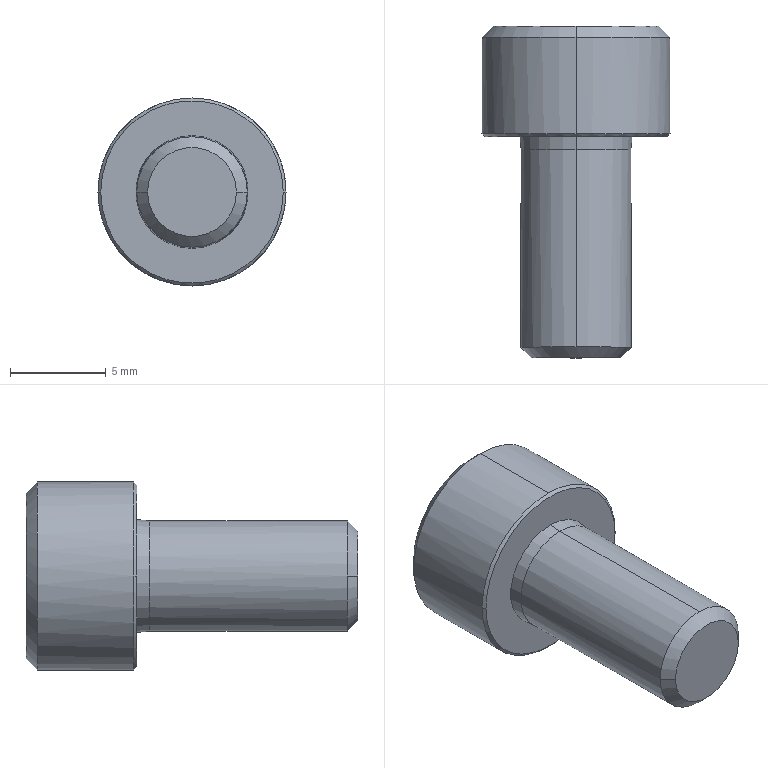Part | SolidWorks | features BaseBody 1 | 1 solid | 36 faces | box 9.808 x 17.308 x 9.808 mm | volume 668.703 mm3 | cone 17 | plane 15 | cylinder 4 | commonest cylinder face diameters 5.769 x2 9.808 x2
STEP:
#1=CARTESIAN_POINT('',(187.694,195.028,223.717));
#2=VERTEX_POINT('',#1);
#3=CARTESIAN_POINT('',(184.809,195.028,220.832));
#4=VERTEX_POINT('',#3);
#5=CARTESIAN_POINT('',(184.809,195.028,223.717));
#6=DIRECTION('',(0.,1.,0.));
#7=DIRECTION('',(0.,0.,1.));
#8=AXIS2_PLACEMENT_3D('',#5,#6,#7);
#9=CIRCLE('',#8,2.885);
#10=EDGE_CURVE('',#2,#4,#9,.T.);
#11=ORIENTED_EDGE('',*,*,#10,.T.);
#12=CARTESIAN_POINT('',(184.809,205.308,220.832));
#13=VERTEX_POINT('',#12);
#14=CARTESIAN_POINT('',(184.809,194.462,220.832));
#15=DIRECTION('',(0.,1.,0.));
#16=VECTOR('',#15,1000.);
#17=LINE('',#14,#16);
#18=EDGE_CURVE('',#4,#13,#17,.T.);
#19=ORIENTED_EDGE('',*,*,#18,.T.);
#20=CARTESIAN_POINT('',(184.809,205.308,226.601));
#21=VERTEX_POINT('',#20);
#22=CARTESIAN_POINT('',(184.809,205.308,223.717));
#23=DIRECTION('',(0.,-1.,0.));
#24=DIRECTION('',(0.,0.,1.));
#25=AXIS2_PLACEMENT_3D('',#22,#23,#24);
#26=CIRCLE('',#25,2.885);
#27=EDGE_CURVE('',#13,#21,#26,.T.);
#28=ORIENTED_EDGE('',*,*,#27,.T.);
#29=CARTESIAN_POINT('',(184.809,195.028,226.601));
#30=VERTEX_POINT('',#29);
#31=CARTESIAN_POINT('',(184.809,194.462,226.601));
#32=DIRECTION('',(0.,1.,0.));
#33=VECTOR('',#32,1000.);
#34=LINE('',#31,#33);
#35=EDGE_CURVE('',#30,#21,#34,.T.);
#36=ORIENTED_EDGE('',*,*,#35,.F.);
#37=CARTESIAN_POINT('',(184.809,195.028,223.717));
#38=DIRECTION('',(0.,1.,0.));
#39=DIRECTION('',(0.,0.,1.));
#40=AXIS2_PLACEMENT_3D('',#37,#38,#39);
#41=CIRCLE('',#40,2.885);
#42=EDGE_CURVE('',#30,#2,#41,.T.);
#43=ORIENTED_EDGE('',*,*,#42,.T.);
#44=EDGE_LOOP('',(#11,#19,#28,#36,#43));
#45=FACE_OUTER_BOUND('',#44,.T.);
#46=CARTESIAN_POINT('',(184.809,194.462,223.717));
#47=DIRECTION('',(0.,1.,0.));
#48=DIRECTION('',(0.,0.,1.));
#49=AXIS2_PLACEMENT_3D('',#46,#47,#48);
#50=CYLINDRICAL_SURFACE('',#49,2.885);
#51=ADVANCED_FACE('',(#45),#50,.T.);
#52=CARTESIAN_POINT('',(182.491,194.462,223.717));
#53=VERTEX_POINT('',#52);
#54=CARTESIAN_POINT('',(187.128,194.462,223.717));
#55=VERTEX_POINT('',#54);
#56=CARTESIAN_POINT('',(184.809,194.462,223.717));
#57=DIRECTION('',(0.,1.,0.));
#58=DIRECTION('',(-1.,0.,0.));
#59=AXIS2_PLACEMENT_3D('',#56,#57,#58);
#60=CIRCLE('',#59,2.319);
#61=EDGE_CURVE('',#53,#55,#60,.T.);
#62=ORIENTED_EDGE('',*,*,#61,.T.);
#63=CARTESIAN_POINT('',(187.694,195.028,223.717));
#64=DIRECTION('',(0.7071,0.7071,0.));
#65=VECTOR('',#64,1000.);
#66=LINE('',#63,#65);
#67=EDGE_CURVE('',#55,#2,#66,.T.);
#68=ORIENTED_EDGE('',*,*,#67,.T.);
#69=ORIENTED_EDGE('',*,*,#42,.F.);
#70=CARTESIAN_POINT('',(181.925,195.028,223.717));
#71=VERTEX_POINT('',#70);
#72=CARTESIAN_POINT('',(184.809,195.028,223.717));
#73=DIRECTION('',(0.,1.,0.));
#74=DIRECTION('',(0.,0.,1.));
#75=AXIS2_PLACEMENT_3D('',#72,#73,#74);
#76=CIRCLE('',#75,2.885);
#77=EDGE_CURVE('',#71,#30,#76,.T.);
#78=ORIENTED_EDGE('',*,*,#77,.F.);
#79=CARTESIAN_POINT('',(181.925,195.028,223.717));
#80=DIRECTION('',(-0.7071,0.7071,0.));
#81=VECTOR('',#80,1000.);
#82=LINE('',#79,#81);
#83=EDGE_CURVE('',#53,#71,#82,.T.);
#84=ORIENTED_EDGE('',*,*,#83,.F.);
#85=EDGE_LOOP('',(#62,#68,#69,#78,#84));
#86=FACE_OUTER_BOUND('',#85,.T.);
#87=CARTESIAN_POINT('',(184.809,195.028,223.717));
#88=DIRECTION('',(0.,1.,0.));
#89=DIRECTION('',(-1.,0.,0.));
#90=AXIS2_PLACEMENT_3D('',#87,#88,#89);
#91=CONICAL_SURFACE('',#90,2.885,0.7854);
#92=ADVANCED_FACE('',(#86),#91,.T.);
#93=ORIENTED_EDGE('',*,*,#27,.F.);
#94=CARTESIAN_POINT('',(184.809,206.,220.774));
#95=VERTEX_POINT('',#94);
#96=CARTESIAN_POINT('',(184.809,206.,220.774));
#97=DIRECTION('',(0.,0.9965,-0.08305));
#98=VECTOR('',#97,1000.);
#99=LINE('',#96,#98);
#100=EDGE_CURVE('',#13,#95,#99,.T.);
#101=ORIENTED_EDGE('',*,*,#100,.T.);
#102=CARTESIAN_POINT('',(184.809,206.,226.659));
#103=VERTEX_POINT('',#102);
#104=CARTESIAN_POINT('',(184.809,206.,223.717));
#105=DIRECTION('',(0.,-1.,0.));
#106=DIRECTION('',(0.,0.,1.));
#107=AXIS2_PLACEMENT_3D('',#104,#105,#106);
#108=CIRCLE('',#107,2.942);
#109=EDGE_CURVE('',#95,#103,#108,.T.);
#110=ORIENTED_EDGE('',*,*,#109,.T.);
#111=CARTESIAN_POINT('',(184.809,206.,226.659));
#112=DIRECTION('',(0.,0.9965,0.08305));
#113=VECTOR('',#112,1000.);
#114=LINE('',#111,#113);
#115=EDGE_CURVE('',#21,#103,#114,.T.);
#116=ORIENTED_EDGE('',*,*,#115,.F.);
#117=EDGE_LOOP('',(#93,#101,#110,#116));
#118=FACE_OUTER_BOUND('',#117,.T.);
#119=CARTESIAN_POINT('',(184.809,206.,223.717));
#120=DIRECTION('',(0.,1.,0.));
#121=DIRECTION('',(0.,0.,1.));
#122=AXIS2_PLACEMENT_3D('',#119,#120,#121);
#123=CONICAL_SURFACE('',#122,2.942,0.08314);
#124=ADVANCED_FACE('',(#118),#123,.T.);
#125=CARTESIAN_POINT('',(180.05,206.,223.717));
#126=VERTEX_POINT('',#125);
#127=CARTESIAN_POINT('',(189.569,206.,223.717));
#128=VERTEX_POINT('',#127);
#129=CARTESIAN_POINT('',(184.809,206.,223.717));
#130=DIRECTION('',(0.,1.,0.));
#131=DIRECTION('',(-1.,0.,0.));
#132=AXIS2_PLACEMENT_3D('',#129,#130,#131);
#133=CIRCLE('',#132,4.76);
#134=EDGE_CURVE('',#126,#128,#133,.T.);
#135=ORIENTED_EDGE('',*,*,#134,.T.);
#136=CARTESIAN_POINT('',(189.713,206.144,223.717));
#137=VERTEX_POINT('',#136);
#138=CARTESIAN_POINT('',(189.713,206.144,223.717));
#139=DIRECTION('',(0.7071,0.7071,0.));
#140=VECTOR('',#139,1000.);
#141=LINE('',#138,#140);
#142=EDGE_CURVE('',#128,#137,#141,.T.);
#143=ORIENTED_EDGE('',*,*,#142,.T.);
#144=CARTESIAN_POINT('',(184.809,206.144,228.621));
#145=VERTEX_POINT('',#144);
#146=CARTESIAN_POINT('',(184.809,206.144,223.717));
#147=DIRECTION('',(0.,-1.,0.));
#148=DIRECTION('',(0.,0.,-1.));
#149=AXIS2_PLACEMENT_3D('',#146,#147,#148);
#150=CIRCLE('',#149,4.904);
#151=EDGE_CURVE('',#137,#145,#150,.T.);
#152=ORIENTED_EDGE('',*,*,#151,.T.);
#153=CARTESIAN_POINT('',(179.906,206.144,223.717));
#154=VERTEX_POINT('',#153);
#155=CARTESIAN_POINT('',(184.809,206.144,223.717));
#156=DIRECTION('',(0.,-1.,0.));
#157=DIRECTION('',(0.,0.,-1.));
#158=AXIS2_PLACEMENT_3D('',#155,#156,#157);
#159=CIRCLE('',#158,4.904);
#160=EDGE_CURVE('',#145,#154,#159,.T.);
#161=ORIENTED_EDGE('',*,*,#160,.T.);
#162=CARTESIAN_POINT('',(179.906,206.144,223.717));
#163=DIRECTION('',(-0.7071,0.7071,0.));
#164=VECTOR('',#163,1000.);
#165=LINE('',#162,#164);
#166=EDGE_CURVE('',#126,#154,#165,.T.);
#167=ORIENTED_EDGE('',*,*,#166,.F.);
#168=EDGE_LOOP('',(#135,#143,#152,#161,#167));
#169=FACE_OUTER_BOUND('',#168,.T.);
#170=CARTESIAN_POINT('',(184.809,206.144,223.717));
#171=DIRECTION('',(0.,1.,0.));
#172=DIRECTION('',(-1.,0.,0.));
#173=AXIS2_PLACEMENT_3D('',#170,#171,#172);
#174=CONICAL_SURFACE('',#173,4.904,0.7854);
#175=ADVANCED_FACE('',(#169),#174,.T.);
#176=CARTESIAN_POINT('',(184.809,206.144,218.813));
#177=VERTEX_POINT('',#176);
#178=CARTESIAN_POINT('',(184.809,206.144,223.717));
#179=DIRECTION('',(0.,-1.,0.));
#180=DIRECTION('',(0.,0.,-1.));
#181=AXIS2_PLACEMENT_3D('',#178,#179,#180);
#182=CIRCLE('',#181,4.904);
#183=EDGE_CURVE('',#177,#137,#182,.T.);
#184=ORIENTED_EDGE('',*,*,#183,.F.);
#185=CARTESIAN_POINT('',(184.809,211.192,218.813));
#186=VERTEX_POINT('',#185);
#187=CARTESIAN_POINT('',(184.809,194.462,218.813));
#188=DIRECTION('',(0.,1.,0.));
#189=VECTOR('',#188,1000.);
#190=LINE('',#187,#189);
#191=EDGE_CURVE('',#177,#186,#190,.T.);
#192=ORIENTED_EDGE('',*,*,#191,.T.);
#193=CARTESIAN_POINT('',(184.809,211.192,228.621));
#194=VERTEX_POINT('',#193);
#195=CARTESIAN_POINT('',(184.809,211.192,223.717));
#196=DIRECTION('',(0.,-1.,0.));
#197=DIRECTION('',(0.,0.,1.));
#198=AXIS2_PLACEMENT_3D('',#195,#196,#197);
#199=CIRCLE('',#198,4.904);
#200=EDGE_CURVE('',#186,#194,#199,.T.);
#201=ORIENTED_EDGE('',*,*,#200,.T.);
#202=CARTESIAN_POINT('',(184.809,194.462,228.621));
#203=DIRECTION('',(0.,1.,0.));
#204=VECTOR('',#203,1000.);
#205=LINE('',#202,#204);
#206=EDGE_CURVE('',#145,#194,#205,.T.);
#207=ORIENTED_EDGE('',*,*,#206,.F.);
#208=ORIENTED_EDGE('',*,*,#151,.F.);
#209=EDGE_LOOP('',(#184,#192,#201,#207,#208));
#210=FACE_OUTER_BOUND('',#209,.T.);
#211=CARTESIAN_POINT('',(184.809,194.462,223.717));
#212=DIRECTION('',(0.,1.,0.));
#213=DIRECTION('',(0.,0.,1.));
#214=AXIS2_PLACEMENT_3D('',#211,#212,#213);
#215=CYLINDRICAL_SURFACE('',#214,4.904);
#216=ADVANCED_FACE('',(#210),#215,.T.);
#217=CARTESIAN_POINT('',(184.809,211.769,219.39));
#218=VERTEX_POINT('',#217);
#219=CARTESIAN_POINT('',(184.809,211.769,228.044));
#220=VERTEX_POINT('',#219);
#221=CARTESIAN_POINT('',(184.809,211.769,223.717));
#222=DIRECTION('',(0.,-1.,0.));
#223=DIRECTION('',(0.,0.,-1.));
#224=AXIS2_PLACEMENT_3D('',#221,#222,#223);
#225=CIRCLE('',#224,4.327);
#226=EDGE_CURVE('',#218,#220,#225,.T.);
#227=ORIENTED_EDGE('',*,*,#226,.T.);
#228=CARTESIAN_POINT('',(184.809,211.192,228.621));
#229=DIRECTION('',(0.,-0.7071,0.7071));
#230=VECTOR('',#229,1000.);
#231=LINE('',#228,#230);
#232=EDGE_CURVE('',#220,#194,#231,.T.);
#233=ORIENTED_EDGE('',*,*,#232,.T.);
#234=ORIENTED_EDGE('',*,*,#200,.F.);
#235=CARTESIAN_POINT('',(184.809,211.192,218.813));
#236=DIRECTION('',(0.,-0.7071,-0.7071));
#237=VECTOR('',#236,1000.);
#238=LINE('',#235,#237);
#239=EDGE_CURVE('',#218,#186,#238,.T.);
#240=ORIENTED_EDGE('',*,*,#239,.F.);
#241=EDGE_LOOP('',(#227,#233,#234,#240));
#242=FACE_OUTER_BOUND('',#241,.T.);
#243=CARTESIAN_POINT('',(184.809,211.192,223.717));
#244=DIRECTION('',(0.,-1.,0.));
#245=DIRECTION('',(0.,0.,-1.));
#246=AXIS2_PLACEMENT_3D('',#243,#244,#245);
#247=CONICAL_SURFACE('',#246,4.904,0.7854);
#248=ADVANCED_FACE('',(#242),#247,.T.);
#249=CARTESIAN_POINT('',(182.502,211.412,223.717));
#250=VERTEX_POINT('',#249);
#251=CARTESIAN_POINT('',(182.502,211.769,225.049));
#252=VERTEX_POINT('',#251);
#253=CARTESIAN_POINT('',(182.502,211.412,223.717));
#254=CARTESIAN_POINT('',(182.502,211.412,223.949));
#255=CARTESIAN_POINT('',(182.502,211.448,224.176));
#256=CARTESIAN_POINT('',(182.502,211.575,224.626));
#257=CARTESIAN_POINT('',(182.502,211.665,224.84));
#258=CARTESIAN_POINT('',(182.502,211.769,225.049));
#259=B_SPLINE_CURVE_WITH_KNOTS('',3,(#253,#254,#255,#256,#257,#258),.UNSPECIFIED.,.F.,.F.,(4,2,4),(0.001381,0.002067,0.002753),.UNSPECIFIED.);
#260=EDGE_CURVE('',#250,#252,#259,.T.);
#261=ORIENTED_EDGE('',*,*,#260,.F.);
#262=CARTESIAN_POINT('',(182.145,211.769,223.717));
#263=VERTEX_POINT('',#262);
#264=CARTESIAN_POINT('',(182.145,211.769,223.717));
#265=DIRECTION('',(-0.7071,0.7071,0.));
#266=VECTOR('',#265,1000.);
#267=LINE('',#264,#266);
#268=EDGE_CURVE('',#250,#263,#267,.T.);
#269=ORIENTED_EDGE('',*,*,#268,.T.);
#270=CARTESIAN_POINT('',(184.809,211.769,223.717));
#271=DIRECTION('',(0.,1.,0.));
#272=DIRECTION('',(-1.,0.,0.));
#273=AXIS2_PLACEMENT_3D('',#270,#271,#272);
#274=CIRCLE('',#273,2.665);
#275=EDGE_CURVE('',#263,#252,#274,.T.);
#276=ORIENTED_EDGE('',*,*,#275,.T.);
#277=EDGE_LOOP('',(#261,#269,#276));
#278=FACE_OUTER_BOUND('',#277,.T.);
#279=CARTESIAN_POINT('',(184.809,211.769,223.717));
#280=DIRECTION('',(0.,1.,0.));
#281=DIRECTION('',(-1.,0.,0.));
#282=AXIS2_PLACEMENT_3D('',#279,#280,#281);
#283=CONICAL_SURFACE('',#282,2.665,0.7854);
#284=ADVANCED_FACE('',(#278),#283,.F.);
#285=CARTESIAN_POINT('',(184.809,207.552,223.717));
#286=VERTEX_POINT('',#285);
#287=CARTESIAN_POINT('',(182.502,208.885,223.717));
#288=VERTEX_POINT('',#287);
#289=CARTESIAN_POINT('',(182.502,208.885,223.717));
#290=DIRECTION('',(-0.866,0.5,0.));
#291=VECTOR('',#290,1000.);
#292=LINE('',#289,#291);
#293=EDGE_CURVE('',#286,#288,#292,.T.);
#294=ORIENTED_EDGE('',*,*,#293,.F.);
#295=CARTESIAN_POINT('',(187.117,208.885,223.717));
#296=VERTEX_POINT('',#295);
#297=CARTESIAN_POINT('',(187.117,208.885,223.717));
#298=DIRECTION('',(0.866,0.5,0.));
#299=VECTOR('',#298,1000.);
#300=LINE('',#297,#299);
#301=EDGE_CURVE('',#286,#296,#300,.T.);
#302=ORIENTED_EDGE('',*,*,#301,.T.);
#303=CARTESIAN_POINT('',(185.963,208.885,221.718));
#304=VERTEX_POINT('',#303);
#305=CARTESIAN_POINT('',(184.809,208.885,223.717));
#306=DIRECTION('',(0.,-1.,0.));
#307=DIRECTION('',(-1.,0.,0.));
#308=AXIS2_PLACEMENT_3D('',#305,#306,#307);
#309=CIRCLE('',#308,2.308);
#310=EDGE_CURVE('',#304,#296,#309,.T.);
#311=ORIENTED_EDGE('',*,*,#310,.F.);
#312=CARTESIAN_POINT('',(183.656,208.885,221.718));
#313=VERTEX_POINT('',#312);
#314=CARTESIAN_POINT('',(184.809,208.885,223.717));
#315=DIRECTION('',(0.,-1.,0.));
#316=DIRECTION('',(-1.,0.,0.));
#317=AXIS2_PLACEMENT_3D('',#314,#315,#316);
#318=CIRCLE('',#317,2.308);
#319=EDGE_CURVE('',#313,#304,#318,.T.);
#320=ORIENTED_EDGE('',*,*,#319,.F.);
#321=CARTESIAN_POINT('',(184.809,208.885,223.717));
#322=DIRECTION('',(0.,-1.,0.));
#323=DIRECTION('',(0.,0.,1.));
#324=AXIS2_PLACEMENT_3D('',#321,#322,#323);
#325=CIRCLE('',#324,2.308);
#326=EDGE_CURVE('',#288,#313,#325,.T.);
#327=ORIENTED_EDGE('',*,*,#326,.F.);
#328=EDGE_LOOP('',(#294,#302,#311,#320,#327));
#329=FACE_OUTER_BOUND('',#328,.T.);
#330=CARTESIAN_POINT('',(184.809,208.885,223.717));
#331=DIRECTION('',(0.,1.,0.));
#332=DIRECTION('',(-1.,0.,0.));
#333=AXIS2_PLACEMENT_3D('',#330,#331,#332);
#334=CONICAL_SURFACE('',#333,2.308,1.047);
#335=ADVANCED_FACE('',(#329),#334,.F.);
#336=ORIENTED_EDGE('',*,*,#18,.F.);
#337=CARTESIAN_POINT('',(184.809,195.028,223.717));
#338=DIRECTION('',(0.,1.,0.));
#339=DIRECTION('',(0.,0.,1.));
#340=AXIS2_PLACEMENT_3D('',#337,#338,#339);
#341=CIRCLE('',#340,2.885);
#342=EDGE_CURVE('',#4,#71,#341,.T.);
#343=ORIENTED_EDGE('',*,*,#342,.T.);
#344=ORIENTED_EDGE('',*,*,#77,.T.);
#345=ORIENTED_EDGE('',*,*,#35,.T.);
#346=CARTESIAN_POINT('',(184.809,205.308,223.717));
#347=DIRECTION('',(0.,-1.,0.));
#348=DIRECTION('',(0.,0.,1.));
#349=AXIS2_PLACEMENT_3D('',#346,#347,#348);
#350=CIRCLE('',#349,2.885);
#351=EDGE_CURVE('',#21,#13,#350,.T.);
#352=ORIENTED_EDGE('',*,*,#351,.T.);
#353=EDGE_LOOP('',(#336,#343,#344,#345,#352));
#354=FACE_OUTER_BOUND('',#353,.T.);
#355=CARTESIAN_POINT('',(184.809,194.462,223.717));
#356=DIRECTION('',(0.,1.,0.));
#357=DIRECTION('',(0.,0.,1.));
#358=AXIS2_PLACEMENT_3D('',#355,#356,#357);
#359=CYLINDRICAL_SURFACE('',#358,2.885);
#360=ADVANCED_FACE('',(#354),#359,.T.);
#361=ORIENTED_EDGE('',*,*,#67,.F.);
#362=CARTESIAN_POINT('',(184.809,194.462,223.717));
#363=DIRECTION('',(0.,1.,0.));
#364=DIRECTION('',(-1.,0.,0.));
#365=AXIS2_PLACEMENT_3D('',#362,#363,#364);
#366=CIRCLE('',#365,2.319);
#367=EDGE_CURVE('',#55,#53,#366,.T.);
#368=ORIENTED_EDGE('',*,*,#367,.T.);
#369=ORIENTED_EDGE('',*,*,#83,.T.);
#370=ORIENTED_EDGE('',*,*,#342,.F.);
#371=ORIENTED_EDGE('',*,*,#10,.F.);
#372=EDGE_LOOP('',(#361,#368,#369,#370,#371));
#373=FACE_OUTER_BOUND('',#372,.T.);
#374=CARTESIAN_POINT('',(184.809,195.028,223.717));
#375=DIRECTION('',(0.,1.,0.));
#376=DIRECTION('',(-1.,0.,0.));
#377=AXIS2_PLACEMENT_3D('',#374,#375,#376);
#378=CONICAL_SURFACE('',#377,2.885,0.7854);
#379=ADVANCED_FACE('',(#373),#378,.T.);
#380=ORIENTED_EDGE('',*,*,#100,.F.);
#381=ORIENTED_EDGE('',*,*,#351,.F.);
#382=ORIENTED_EDGE('',*,*,#115,.T.);
#383=CARTESIAN_POINT('',(184.809,206.,223.717));
#384=DIRECTION('',(0.,-1.,0.));
#385=DIRECTION('',(0.,0.,1.));
#386=AXIS2_PLACEMENT_3D('',#383,#384,#385);
#387=CIRCLE('',#386,2.942);
#388=EDGE_CURVE('',#103,#95,#387,.T.);
#389=ORIENTED_EDGE('',*,*,#388,.T.);
#390=EDGE_LOOP('',(#380,#381,#382,#389));
#391=FACE_OUTER_BOUND('',#390,.T.);
#392=CARTESIAN_POINT('',(184.809,206.,223.717));
#393=DIRECTION('',(0.,1.,0.));
#394=DIRECTION('',(0.,0.,1.));
#395=AXIS2_PLACEMENT_3D('',#392,#393,#394);
#396=CONICAL_SURFACE('',#395,2.942,0.08314);
#397=ADVANCED_FACE('',(#391),#396,.T.);
#398=ORIENTED_EDGE('',*,*,#61,.F.);
#399=ORIENTED_EDGE('',*,*,#367,.F.);
#400=EDGE_LOOP('',(#398,#399));
#401=FACE_OUTER_BOUND('',#400,.T.);
#402=CARTESIAN_POINT('',(187.128,194.462,223.717));
#403=DIRECTION('',(0.,1.,0.));
#404=DIRECTION('',(0.,0.,1.));
#405=AXIS2_PLACEMENT_3D('',#402,#403,#404);
#406=PLANE('',#405);
#407=ADVANCED_FACE('',(#401),#406,.F.);
#408=ORIENTED_EDGE('',*,*,#388,.F.);
#409=ORIENTED_EDGE('',*,*,#109,.F.);
#410=EDGE_LOOP('',(#408,#409));
#411=FACE_BOUND('',#410,.T.);
#412=ORIENTED_EDGE('',*,*,#134,.F.);
#413=CARTESIAN_POINT('',(184.809,206.,223.717));
#414=DIRECTION('',(0.,1.,0.));
#415=DIRECTION('',(-1.,0.,0.));
#416=AXIS2_PLACEMENT_3D('',#413,#414,#415);
#417=CIRCLE('',#416,4.76);
#418=EDGE_CURVE('',#128,#126,#417,.T.);
#419=ORIENTED_EDGE('',*,*,#418,.F.);
#420=EDGE_LOOP('',(#412,#419));
#421=FACE_OUTER_BOUND('',#420,.T.);
#422=CARTESIAN_POINT('',(189.569,206.,223.717));
#423=DIRECTION('',(0.,1.,0.));
#424=DIRECTION('',(0.,0.,1.));
#425=AXIS2_PLACEMENT_3D('',#422,#423,#424);
#426=PLANE('',#425);
#427=ADVANCED_FACE('',(#411,#421),#426,.F.);
#428=ORIENTED_EDGE('',*,*,#142,.F.);
#429=ORIENTED_EDGE('',*,*,#418,.T.);
#430=ORIENTED_EDGE('',*,*,#166,.T.);
#431=CARTESIAN_POINT('',(184.809,206.144,223.717));
#432=DIRECTION('',(0.,-1.,0.));
#433=DIRECTION('',(0.,0.,-1.));
#434=AXIS2_PLACEMENT_3D('',#431,#432,#433);
#435=CIRCLE('',#434,4.904);
#436=EDGE_CURVE('',#154,#177,#435,.T.);
#437=ORIENTED_EDGE('',*,*,#436,.T.);
#438=ORIENTED_EDGE('',*,*,#183,.T.);
#439=EDGE_LOOP('',(#428,#429,#430,#437,#438));
#440=FACE_OUTER_BOUND('',#439,.T.);
#441=CARTESIAN_POINT('',(184.809,206.144,223.717));
#442=DIRECTION('',(0.,1.,0.));
#443=DIRECTION('',(-1.,0.,0.));
#444=AXIS2_PLACEMENT_3D('',#441,#442,#443);
#445=CONICAL_SURFACE('',#444,4.904,0.7854);
#446=ADVANCED_FACE('',(#440),#445,.T.);
#447=ORIENTED_EDGE('',*,*,#191,.F.);
#448=ORIENTED_EDGE('',*,*,#436,.F.);
#449=ORIENTED_EDGE('',*,*,#160,.F.);
#450=ORIENTED_EDGE('',*,*,#206,.T.);
#451=CARTESIAN_POINT('',(184.809,211.192,223.717));
#452=DIRECTION('',(0.,-1.,0.));
#453=DIRECTION('',(0.,0.,1.));
#454=AXIS2_PLACEMENT_3D('',#451,#452,#453);
#455=CIRCLE('',#454,4.904);
#456=EDGE_CURVE('',#194,#186,#455,.T.);
#457=ORIENTED_EDGE('',*,*,#456,.T.);
#458=EDGE_LOOP('',(#447,#448,#449,#450,#457));
#459=FACE_OUTER_BOUND('',#458,.T.);
#460=CARTESIAN_POINT('',(184.809,194.462,223.717));
#461=DIRECTION('',(0.,1.,0.));
#462=DIRECTION('',(0.,0.,1.));
#463=AXIS2_PLACEMENT_3D('',#460,#461,#462);
#464=CYLINDRICAL_SURFACE('',#463,4.904);
#465=ADVANCED_FACE('',(#459),#464,.T.);
#466=ORIENTED_EDGE('',*,*,#232,.F.);
#467=CARTESIAN_POINT('',(184.809,211.769,223.717));
#468=DIRECTION('',(0.,-1.,0.));
#469=DIRECTION('',(0.,0.,-1.));
#470=AXIS2_PLACEMENT_3D('',#467,#468,#469);
#471=CIRCLE('',#470,4.327);
#472=EDGE_CURVE('',#220,#218,#471,.T.);
#473=ORIENTED_EDGE('',*,*,#472,.T.);
#474=ORIENTED_EDGE('',*,*,#239,.T.);
#475=ORIENTED_EDGE('',*,*,#456,.F.);
#476=EDGE_LOOP('',(#466,#473,#474,#475));
#477=FACE_OUTER_BOUND('',#476,.T.);
#478=CARTESIAN_POINT('',(184.809,211.192,223.717));
#479=DIRECTION('',(0.,-1.,0.));
#480=DIRECTION('',(0.,0.,-1.));
#481=AXIS2_PLACEMENT_3D('',#478,#479,#480);
#482=CONICAL_SURFACE('',#481,4.904,0.7854);
#483=ADVANCED_FACE('',(#477),#482,.T.);
#484=CARTESIAN_POINT('',(184.809,211.769,226.381));
#485=VERTEX_POINT('',#484);
#486=CARTESIAN_POINT('',(184.809,211.769,223.717));
#487=DIRECTION('',(0.,1.,0.));
#488=DIRECTION('',(-1.,0.,0.));
#489=AXIS2_PLACEMENT_3D('',#486,#487,#488);
#490=CIRCLE('',#489,2.665);
#491=EDGE_CURVE('',#252,#485,#490,.T.);
#492=ORIENTED_EDGE('',*,*,#491,.F.);
#493=ORIENTED_EDGE('',*,*,#275,.F.);
#494=CARTESIAN_POINT('',(182.502,211.769,222.384));
#495=VERTEX_POINT('',#494);
#496=CARTESIAN_POINT('',(184.809,211.769,223.717));
#497=DIRECTION('',(0.,1.,0.));
#498=DIRECTION('',(-1.,0.,0.));
#499=AXIS2_PLACEMENT_3D('',#496,#497,#498);
#500=CIRCLE('',#499,2.665);
#501=EDGE_CURVE('',#495,#263,#500,.T.);
#502=ORIENTED_EDGE('',*,*,#501,.F.);
#503=CARTESIAN_POINT('',(184.809,211.769,221.052));
#504=VERTEX_POINT('',#503);
#505=CARTESIAN_POINT('',(184.809,211.769,223.717));
#506=DIRECTION('',(0.,1.,0.));
#507=DIRECTION('',(0.,0.,1.));
#508=AXIS2_PLACEMENT_3D('',#505,#506,#507);
#509=CIRCLE('',#508,2.665);
#510=EDGE_CURVE('',#504,#495,#509,.T.);
#511=ORIENTED_EDGE('',*,*,#510,.F.);
#512=CARTESIAN_POINT('',(187.117,211.769,222.384));
#513=VERTEX_POINT('',#512);
#514=CARTESIAN_POINT('',(184.809,211.769,223.717));
#515=DIRECTION('',(0.,1.,0.));
#516=DIRECTION('',(0.,0.,1.));
#517=AXIS2_PLACEMENT_3D('',#514,#515,#516);
#518=CIRCLE('',#517,2.665);
#519=EDGE_CURVE('',#513,#504,#518,.T.);
#520=ORIENTED_EDGE('',*,*,#519,.F.);
#521=CARTESIAN_POINT('',(187.117,211.769,225.049));
#522=VERTEX_POINT('',#521);
#523=CARTESIAN_POINT('',(184.809,211.769,223.717));
#524=DIRECTION('',(0.,1.,0.));
#525=DIRECTION('',(0.,0.,1.));
#526=AXIS2_PLACEMENT_3D('',#523,#524,#525);
#527=CIRCLE('',#526,2.665);
#528=EDGE_CURVE('',#522,#513,#527,.T.);
#529=ORIENTED_EDGE('',*,*,#528,.F.);
#530=CARTESIAN_POINT('',(184.809,211.769,223.717));
#531=DIRECTION('',(0.,1.,0.));
#532=DIRECTION('',(0.,0.,1.));
#533=AXIS2_PLACEMENT_3D('',#530,#531,#532);
#534=CIRCLE('',#533,2.665);
#535=EDGE_CURVE('',#485,#522,#534,.T.);
#536=ORIENTED_EDGE('',*,*,#535,.F.);
#537=EDGE_LOOP('',(#492,#493,#502,#511,#520,#529,#536));
#538=FACE_BOUND('',#537,.T.);
#539=ORIENTED_EDGE('',*,*,#226,.F.);
#540=ORIENTED_EDGE('',*,*,#472,.F.);
#541=EDGE_LOOP('',(#539,#540));
#542=FACE_OUTER_BOUND('',#541,.T.);
#543=CARTESIAN_POINT('',(187.474,211.769,223.717));
#544=DIRECTION('',(0.,-1.,0.));
#545=DIRECTION('',(0.,0.,-1.));
#546=AXIS2_PLACEMENT_3D('',#543,#544,#545);
#547=PLANE('',#546);
#548=ADVANCED_FACE('',(#538,#542),#547,.F.);
#549=CARTESIAN_POINT('',(184.809,211.769,226.381));
#550=CARTESIAN_POINT('',(184.99,211.665,226.277));
#551=CARTESIAN_POINT('',(185.174,211.577,226.171));
#552=CARTESIAN_POINT('',(185.461,211.482,226.006));
#553=CARTESIAN_POINT('',(185.558,211.457,225.949));
#554=CARTESIAN_POINT('',(185.756,211.422,225.835));
#555=CARTESIAN_POINT('',(185.858,211.413,225.776));
#556=CARTESIAN_POINT('',(186.161,211.412,225.601));
#557=CARTESIAN_POINT('',(186.359,211.447,225.487));
#558=CARTESIAN_POINT('',(186.749,211.575,225.262));
#559=CARTESIAN_POINT('',(186.936,211.665,225.154));
#560=CARTESIAN_POINT('',(187.117,211.769,225.049));
#561=B_SPLINE_CURVE_WITH_KNOTS('',3,(#549,#550,#551,#552,#553,#554,#555,#556,#557,#558,#559,#560),.UNSPECIFIED.,.F.,.F.,(4,2,2,2,2,4),(0.,0.0006881,0.001032,0.001376,0.002064,0.002753),.UNSPECIFIED.);
#562=EDGE_CURVE('',#485,#522,#561,.T.);
#563=ORIENTED_EDGE('',*,*,#562,.F.);
#564=ORIENTED_EDGE('',*,*,#535,.T.);
#565=EDGE_LOOP('',(#563,#564));
#566=FACE_OUTER_BOUND('',#565,.T.);
#567=CARTESIAN_POINT('',(184.809,211.769,223.717));
#568=DIRECTION('',(0.,1.,0.));
#569=DIRECTION('',(0.,0.,1.));
#570=AXIS2_PLACEMENT_3D('',#567,#568,#569);
#571=CONICAL_SURFACE('',#570,2.665,0.7854);
#572=ADVANCED_FACE('',(#566),#571,.F.);
#573=CARTESIAN_POINT('',(182.502,211.769,225.049));
#574=CARTESIAN_POINT('',(182.682,211.665,225.153));
#575=CARTESIAN_POINT('',(182.866,211.577,225.26));
#576=CARTESIAN_POINT('',(183.153,211.482,225.425));
#577=CARTESIAN_POINT('',(183.25,211.457,225.481));
#578=CARTESIAN_POINT('',(183.448,211.422,225.596));
#579=CARTESIAN_POINT('',(183.551,211.413,225.655));
#580=CARTESIAN_POINT('',(183.853,211.412,225.829));
#581=CARTESIAN_POINT('',(184.051,211.447,225.944));
#582=CARTESIAN_POINT('',(184.441,211.575,226.169));
#583=CARTESIAN_POINT('',(184.628,211.665,226.277));
#584=CARTESIAN_POINT('',(184.809,211.769,226.381));
#585=B_SPLINE_CURVE_WITH_KNOTS('',3,(#573,#574,#575,#576,#577,#578,#579,#580,#581,#582,#583,#584),.UNSPECIFIED.,.F.,.F.,(4,2,2,2,2,4),(0.,0.0006881,0.001032,0.001376,0.002064,0.002753),.UNSPECIFIED.);
#586=EDGE_CURVE('',#252,#485,#585,.T.);
#587=ORIENTED_EDGE('',*,*,#586,.F.);
#588=ORIENTED_EDGE('',*,*,#491,.T.);
#589=EDGE_LOOP('',(#587,#588));
#590=FACE_OUTER_BOUND('',#589,.T.);
#591=CARTESIAN_POINT('',(184.809,211.769,223.717));
#592=DIRECTION('',(0.,1.,0.));
#593=DIRECTION('',(-1.,0.,0.));
#594=AXIS2_PLACEMENT_3D('',#591,#592,#593);
#595=CONICAL_SURFACE('',#594,2.665,0.7854);
#596=ADVANCED_FACE('',(#590),#595,.F.);
#597=ORIENTED_EDGE('',*,*,#268,.F.);
#598=CARTESIAN_POINT('',(182.502,211.769,222.384));
#599=CARTESIAN_POINT('',(182.502,211.665,222.593));
#600=CARTESIAN_POINT('',(182.502,211.576,222.807));
#601=CARTESIAN_POINT('',(182.502,211.481,223.139));
#602=CARTESIAN_POINT('',(182.502,211.456,223.252));
#603=CARTESIAN_POINT('',(182.502,211.421,223.482));
#604=CARTESIAN_POINT('',(182.502,211.412,223.6));
#605=CARTESIAN_POINT('',(182.502,211.412,223.717));
#606=B_SPLINE_CURVE_WITH_KNOTS('',3,(#598,#599,#600,#601,#602,#603,#604,#605),.UNSPECIFIED.,.F.,.F.,(4,2,2,4),(0.,0.0006905,0.001036,0.001381),.UNSPECIFIED.);
#607=EDGE_CURVE('',#495,#250,#606,.T.);
#608=ORIENTED_EDGE('',*,*,#607,.F.);
#609=ORIENTED_EDGE('',*,*,#501,.T.);
#610=EDGE_LOOP('',(#597,#608,#609));
#611=FACE_OUTER_BOUND('',#610,.T.);
#612=CARTESIAN_POINT('',(184.809,211.769,223.717));
#613=DIRECTION('',(0.,1.,0.));
#614=DIRECTION('',(-1.,0.,0.));
#615=AXIS2_PLACEMENT_3D('',#612,#613,#614);
#616=CONICAL_SURFACE('',#615,2.665,0.7854);
#617=ADVANCED_FACE('',(#611),#616,.F.);
#618=CARTESIAN_POINT('',(184.809,211.769,221.052));
#619=CARTESIAN_POINT('',(184.629,211.665,221.156));
#620=CARTESIAN_POINT('',(184.445,211.577,221.263));
#621=CARTESIAN_POINT('',(184.158,211.482,221.428));
#622=CARTESIAN_POINT('',(184.061,211.457,221.484));
#623=CARTESIAN_POINT('',(183.863,211.422,221.599));
#624=CARTESIAN_POINT('',(183.761,211.413,221.658));
#625=CARTESIAN_POINT('',(183.458,211.412,221.832));
#626=CARTESIAN_POINT('',(183.26,211.447,221.946));
#627=CARTESIAN_POINT('',(182.87,211.575,222.172));
#628=CARTESIAN_POINT('',(182.683,211.665,222.28));
#629=CARTESIAN_POINT('',(182.502,211.769,222.384));
#630=B_SPLINE_CURVE_WITH_KNOTS('',3,(#618,#619,#620,#621,#622,#623,#624,#625,#626,#627,#628,#629),.UNSPECIFIED.,.F.,.F.,(4,2,2,2,2,4),(0.,0.0006881,0.001032,0.001376,0.002064,0.002753),.UNSPECIFIED.);
#631=EDGE_CURVE('',#504,#495,#630,.T.);
#632=ORIENTED_EDGE('',*,*,#631,.F.);
#633=ORIENTED_EDGE('',*,*,#510,.T.);
#634=EDGE_LOOP('',(#632,#633));
#635=FACE_OUTER_BOUND('',#634,.T.);
#636=CARTESIAN_POINT('',(184.809,211.769,223.717));
#637=DIRECTION('',(0.,1.,0.));
#638=DIRECTION('',(0.,0.,1.));
#639=AXIS2_PLACEMENT_3D('',#636,#637,#638);
#640=CONICAL_SURFACE('',#639,2.665,0.7854);
#641=ADVANCED_FACE('',(#635),#640,.F.);
#642=CARTESIAN_POINT('',(187.117,211.769,222.384));
#643=CARTESIAN_POINT('',(186.937,211.665,222.28));
#644=CARTESIAN_POINT('',(186.752,211.577,222.174));
#645=CARTESIAN_POINT('',(186.466,211.482,222.009));
#646=CARTESIAN_POINT('',(186.369,211.457,221.952));
#647=CARTESIAN_POINT('',(186.17,211.422,221.838));
#648=CARTESIAN_POINT('',(186.068,211.413,221.779));
#649=CARTESIAN_POINT('',(185.766,211.412,221.604));
#650=CARTESIAN_POINT('',(185.568,211.447,221.49));
#651=CARTESIAN_POINT('',(185.178,211.575,221.265));
#652=CARTESIAN_POINT('',(184.991,211.665,221.157));
#653=CARTESIAN_POINT('',(184.809,211.769,221.052));
#654=B_SPLINE_CURVE_WITH_KNOTS('',3,(#642,#643,#644,#645,#646,#647,#648,#649,#650,#651,#652,#653),.UNSPECIFIED.,.F.,.F.,(4,2,2,2,2,4),(0.,0.0006881,0.001032,0.001376,0.002064,0.002753),.UNSPECIFIED.);
#655=EDGE_CURVE('',#513,#504,#654,.T.);
#656=ORIENTED_EDGE('',*,*,#655,.F.);
#657=ORIENTED_EDGE('',*,*,#519,.T.);
#658=EDGE_LOOP('',(#656,#657));
#659=FACE_OUTER_BOUND('',#658,.T.);
#660=CARTESIAN_POINT('',(184.809,211.769,223.717));
#661=DIRECTION('',(0.,1.,0.));
#662=DIRECTION('',(0.,0.,1.));
#663=AXIS2_PLACEMENT_3D('',#660,#661,#662);
#664=CONICAL_SURFACE('',#663,2.665,0.7854);
#665=ADVANCED_FACE('',(#659),#664,.F.);
#666=CARTESIAN_POINT('',(187.117,211.769,225.049));
#667=CARTESIAN_POINT('',(187.117,211.665,224.841));
#668=CARTESIAN_POINT('',(187.117,211.577,224.628));
#669=CARTESIAN_POINT('',(187.117,211.482,224.297));
#670=CARTESIAN_POINT('',(187.117,211.457,224.185));
#671=CARTESIAN_POINT('',(187.117,211.422,223.956));
#672=CARTESIAN_POINT('',(187.117,211.413,223.838));
#673=CARTESIAN_POINT('',(187.117,211.412,223.489));
#674=CARTESIAN_POINT('',(187.117,211.447,223.26));
#675=CARTESIAN_POINT('',(187.117,211.575,222.81));
#676=CARTESIAN_POINT('',(187.117,211.665,222.594));
#677=CARTESIAN_POINT('',(187.117,211.769,222.384));
#678=B_SPLINE_CURVE_WITH_KNOTS('',3,(#666,#667,#668,#669,#670,#671,#672,#673,#674,#675,#676,#677),.UNSPECIFIED.,.F.,.F.,(4,2,2,2,2,4),(0.,0.0006881,0.001032,0.001376,0.002064,0.002753),.UNSPECIFIED.);
#679=EDGE_CURVE('',#522,#513,#678,.T.);
#680=ORIENTED_EDGE('',*,*,#679,.F.);
#681=ORIENTED_EDGE('',*,*,#528,.T.);
#682=EDGE_LOOP('',(#680,#681));
#683=FACE_OUTER_BOUND('',#682,.T.);
#684=CARTESIAN_POINT('',(184.809,211.769,223.717));
#685=DIRECTION('',(0.,1.,0.));
#686=DIRECTION('',(0.,0.,1.));
#687=AXIS2_PLACEMENT_3D('',#684,#685,#686);
#688=CONICAL_SURFACE('',#687,2.665,0.7854);
#689=ADVANCED_FACE('',(#683),#688,.F.);
#690=CARTESIAN_POINT('',(187.117,208.885,225.049));
#691=VERTEX_POINT('',#690);
#692=CARTESIAN_POINT('',(187.117,208.885,225.049));
#693=DIRECTION('',(0.,1.,0.));
#694=VECTOR('',#693,1000.);
#695=LINE('',#692,#694);
#696=EDGE_CURVE('',#691,#522,#695,.T.);
#697=ORIENTED_EDGE('',*,*,#696,.F.);
#698=CARTESIAN_POINT('',(185.963,208.885,225.715));
#699=VERTEX_POINT('',#698);
#700=CARTESIAN_POINT('',(184.809,208.885,226.381));
#701=DIRECTION('',(0.866,0.,-0.5));
#702=VECTOR('',#701,1000.);
#703=LINE('',#700,#702);
#704=EDGE_CURVE('',#699,#691,#703,.T.);
#705=ORIENTED_EDGE('',*,*,#704,.F.);
#706=CARTESIAN_POINT('',(184.809,208.885,226.381));
#707=VERTEX_POINT('',#706);
#708=CARTESIAN_POINT('',(184.809,208.885,226.381));
#709=DIRECTION('',(0.866,0.,-0.5));
#710=VECTOR('',#709,1000.);
#711=LINE('',#708,#710);
#712=EDGE_CURVE('',#707,#699,#711,.T.);
#713=ORIENTED_EDGE('',*,*,#712,.F.);
#714=CARTESIAN_POINT('',(184.809,208.885,226.381));
#715=DIRECTION('',(0.,-1.,0.));
#716=VECTOR('',#715,1000.);
#717=LINE('',#714,#716);
#718=EDGE_CURVE('',#485,#707,#717,.T.);
#719=ORIENTED_EDGE('',*,*,#718,.F.);
#720=ORIENTED_EDGE('',*,*,#562,.T.);
#721=EDGE_LOOP('',(#697,#705,#713,#719,#720));
#722=FACE_OUTER_BOUND('',#721,.T.);
#723=CARTESIAN_POINT('',(184.809,208.885,226.381));
#724=DIRECTION('',(0.5,0.,0.866));
#725=DIRECTION('',(0.866,0.,-0.5));
#726=AXIS2_PLACEMENT_3D('',#723,#724,#725);
#727=PLANE('',#726);
#728=ADVANCED_FACE('',(#722),#727,.F.);
#729=ORIENTED_EDGE('',*,*,#718,.T.);
#730=CARTESIAN_POINT('',(183.656,208.885,225.715));
#731=VERTEX_POINT('',#730);
#732=CARTESIAN_POINT('',(182.502,208.885,225.049));
#733=DIRECTION('',(0.866,0.,0.5));
#734=VECTOR('',#733,1000.);
#735=LINE('',#732,#734);
#736=EDGE_CURVE('',#731,#707,#735,.T.);
#737=ORIENTED_EDGE('',*,*,#736,.F.);
#738=CARTESIAN_POINT('',(182.502,208.885,225.049));
#739=VERTEX_POINT('',#738);
#740=CARTESIAN_POINT('',(182.502,208.885,225.049));
#741=DIRECTION('',(0.866,0.,0.5));
#742=VECTOR('',#741,1000.);
#743=LINE('',#740,#742);
#744=EDGE_CURVE('',#739,#731,#743,.T.);
#745=ORIENTED_EDGE('',*,*,#744,.F.);
#746=CARTESIAN_POINT('',(182.502,208.885,225.049));
#747=DIRECTION('',(0.,-1.,0.));
#748=VECTOR('',#747,1000.);
#749=LINE('',#746,#748);
#750=EDGE_CURVE('',#252,#739,#749,.T.);
#751=ORIENTED_EDGE('',*,*,#750,.F.);
#752=ORIENTED_EDGE('',*,*,#586,.T.);
#753=EDGE_LOOP('',(#729,#737,#745,#751,#752));
#754=FACE_OUTER_BOUND('',#753,.T.);
#755=CARTESIAN_POINT('',(182.502,208.885,225.049));
#756=DIRECTION('',(-0.5,0.,0.866));
#757=DIRECTION('',(0.866,0.,0.5));
#758=AXIS2_PLACEMENT_3D('',#755,#756,#757);
#759=PLANE('',#758);
#760=ADVANCED_FACE('',(#754),#759,.F.);
#761=ORIENTED_EDGE('',*,*,#750,.T.);
#762=CARTESIAN_POINT('',(182.502,208.885,222.384));
#763=DIRECTION('',(0.,0.,1.));
#764=VECTOR('',#763,1000.);
#765=LINE('',#762,#764);
#766=EDGE_CURVE('',#288,#739,#765,.T.);
#767=ORIENTED_EDGE('',*,*,#766,.F.);
#768=CARTESIAN_POINT('',(182.502,208.885,222.384));
#769=VERTEX_POINT('',#768);
#770=CARTESIAN_POINT('',(182.502,208.885,222.384));
#771=DIRECTION('',(0.,0.,1.));
#772=VECTOR('',#771,1000.);
#773=LINE('',#770,#772);
#774=EDGE_CURVE('',#769,#288,#773,.T.);
#775=ORIENTED_EDGE('',*,*,#774,.F.);
#776=CARTESIAN_POINT('',(182.502,208.885,222.384));
#777=DIRECTION('',(0.,-1.,0.));
#778=VECTOR('',#777,1000.);
#779=LINE('',#776,#778);
#780=EDGE_CURVE('',#495,#769,#779,.T.);
#781=ORIENTED_EDGE('',*,*,#780,.F.);
#782=ORIENTED_EDGE('',*,*,#607,.T.);
#783=ORIENTED_EDGE('',*,*,#260,.T.);
#784=EDGE_LOOP('',(#761,#767,#775,#781,#782,#783));
#785=FACE_OUTER_BOUND('',#784,.T.);
#786=CARTESIAN_POINT('',(182.502,208.885,222.384));
#787=DIRECTION('',(-1.,0.,0.));
#788=DIRECTION('',(0.,0.,1.));
#789=AXIS2_PLACEMENT_3D('',#786,#787,#788);
#790=PLANE('',#789);
#791=ADVANCED_FACE('',(#785),#790,.F.);
#792=ORIENTED_EDGE('',*,*,#780,.T.);
#793=CARTESIAN_POINT('',(184.809,208.885,221.052));
#794=DIRECTION('',(-0.866,0.,0.5));
#795=VECTOR('',#794,1000.);
#796=LINE('',#793,#795);
#797=EDGE_CURVE('',#313,#769,#796,.T.);
#798=ORIENTED_EDGE('',*,*,#797,.F.);
#799=CARTESIAN_POINT('',(184.809,208.885,221.052));
#800=VERTEX_POINT('',#799);
#801=CARTESIAN_POINT('',(184.809,208.885,221.052));
#802=DIRECTION('',(-0.866,0.,0.5));
#803=VECTOR('',#802,1000.);
#804=LINE('',#801,#803);
#805=EDGE_CURVE('',#800,#313,#804,.T.);
#806=ORIENTED_EDGE('',*,*,#805,.F.);
#807=CARTESIAN_POINT('',(184.809,208.885,221.052));
#808=DIRECTION('',(0.,-1.,0.));
#809=VECTOR('',#808,1000.);
#810=LINE('',#807,#809);
#811=EDGE_CURVE('',#504,#800,#810,.T.);
#812=ORIENTED_EDGE('',*,*,#811,.F.);
#813=ORIENTED_EDGE('',*,*,#631,.T.);
#814=EDGE_LOOP('',(#792,#798,#806,#812,#813));
#815=FACE_OUTER_BOUND('',#814,.T.);
#816=CARTESIAN_POINT('',(184.809,208.885,221.052));
#817=DIRECTION('',(-0.5,0.,-0.866));
#818=DIRECTION('',(-0.866,0.,0.5));
#819=AXIS2_PLACEMENT_3D('',#816,#817,#818);
#820=PLANE('',#819);
#821=ADVANCED_FACE('',(#815),#820,.F.);
#822=ORIENTED_EDGE('',*,*,#811,.T.);
#823=CARTESIAN_POINT('',(187.117,208.885,222.384));
#824=DIRECTION('',(-0.866,0.,-0.5));
#825=VECTOR('',#824,1000.);
#826=LINE('',#823,#825);
#827=EDGE_CURVE('',#304,#800,#826,.T.);
#828=ORIENTED_EDGE('',*,*,#827,.F.);
#829=CARTESIAN_POINT('',(187.117,208.885,222.384));
#830=VERTEX_POINT('',#829);
#831=CARTESIAN_POINT('',(187.117,208.885,222.384));
#832=DIRECTION('',(-0.866,0.,-0.5));
#833=VECTOR('',#832,1000.);
#834=LINE('',#831,#833);
#835=EDGE_CURVE('',#830,#304,#834,.T.);
#836=ORIENTED_EDGE('',*,*,#835,.F.);
#837=CARTESIAN_POINT('',(187.117,208.885,222.384));
#838=DIRECTION('',(0.,-1.,0.));
#839=VECTOR('',#838,1000.);
#840=LINE('',#837,#839);
#841=EDGE_CURVE('',#513,#830,#840,.T.);
#842=ORIENTED_EDGE('',*,*,#841,.F.);
#843=ORIENTED_EDGE('',*,*,#655,.T.);
#844=EDGE_LOOP('',(#822,#828,#836,#842,#843));
#845=FACE_OUTER_BOUND('',#844,.T.);
#846=CARTESIAN_POINT('',(187.117,208.885,222.384));
#847=DIRECTION('',(0.5,0.,-0.866));
#848=DIRECTION('',(-0.866,0.,-0.5));
#849=AXIS2_PLACEMENT_3D('',#846,#847,#848);
#850=PLANE('',#849);
#851=ADVANCED_FACE('',(#845),#850,.F.);
#852=ORIENTED_EDGE('',*,*,#841,.T.);
#853=CARTESIAN_POINT('',(187.117,208.885,225.049));
#854=DIRECTION('',(0.,0.,-1.));
#855=VECTOR('',#854,1000.);
#856=LINE('',#853,#855);
#857=EDGE_CURVE('',#296,#830,#856,.T.);
#858=ORIENTED_EDGE('',*,*,#857,.F.);
#859=CARTESIAN_POINT('',(187.117,208.885,225.049));
#860=DIRECTION('',(0.,0.,-1.));
#861=VECTOR('',#860,1000.);
#862=LINE('',#859,#861);
#863=EDGE_CURVE('',#691,#296,#862,.T.);
#864=ORIENTED_EDGE('',*,*,#863,.F.);
#865=ORIENTED_EDGE('',*,*,#696,.T.);
#866=ORIENTED_EDGE('',*,*,#679,.T.);
#867=EDGE_LOOP('',(#852,#858,#864,#865,#866));
#868=FACE_OUTER_BOUND('',#867,.T.);
#869=CARTESIAN_POINT('',(187.117,208.885,225.049));
#870=DIRECTION('',(1.,0.,0.));
#871=DIRECTION('',(0.,0.,-1.));
#872=AXIS2_PLACEMENT_3D('',#869,#870,#871);
#873=PLANE('',#872);
#874=ADVANCED_FACE('',(#868),#873,.F.);
#875=CARTESIAN_POINT('',(184.809,208.885,223.717));
#876=DIRECTION('',(0.,-1.,0.));
#877=DIRECTION('',(-1.,0.,0.));
#878=AXIS2_PLACEMENT_3D('',#875,#876,#877);
#879=CIRCLE('',#878,2.308);
#880=EDGE_CURVE('',#296,#699,#879,.T.);
#881=ORIENTED_EDGE('',*,*,#880,.T.);
#882=ORIENTED_EDGE('',*,*,#704,.T.);
#883=ORIENTED_EDGE('',*,*,#863,.T.);
#884=EDGE_LOOP('',(#881,#882,#883));
#885=FACE_OUTER_BOUND('',#884,.T.);
#886=CARTESIAN_POINT('',(184.809,208.885,223.717));
#887=DIRECTION('',(0.,1.,0.));
#888=DIRECTION('',(0.,0.,1.));
#889=AXIS2_PLACEMENT_3D('',#886,#887,#888);
#890=PLANE('',#889);
#891=ADVANCED_FACE('',(#885),#890,.T.);
#892=CARTESIAN_POINT('',(184.809,208.885,223.717));
#893=DIRECTION('',(0.,-1.,0.));
#894=DIRECTION('',(0.,0.,1.));
#895=AXIS2_PLACEMENT_3D('',#892,#893,#894);
#896=CIRCLE('',#895,2.308);
#897=EDGE_CURVE('',#699,#731,#896,.T.);
#898=ORIENTED_EDGE('',*,*,#897,.T.);
#899=ORIENTED_EDGE('',*,*,#736,.T.);
#900=ORIENTED_EDGE('',*,*,#712,.T.);
#901=EDGE_LOOP('',(#898,#899,#900));
#902=FACE_OUTER_BOUND('',#901,.T.);
#903=CARTESIAN_POINT('',(184.809,208.885,223.717));
#904=DIRECTION('',(0.,1.,0.));
#905=DIRECTION('',(0.,0.,1.));
#906=AXIS2_PLACEMENT_3D('',#903,#904,#905);
#907=PLANE('',#906);
#908=ADVANCED_FACE('',(#902),#907,.T.);
#909=CARTESIAN_POINT('',(184.809,208.885,223.717));
#910=DIRECTION('',(0.,-1.,0.));
#911=DIRECTION('',(0.,0.,1.));
#912=AXIS2_PLACEMENT_3D('',#909,#910,#911);
#913=CIRCLE('',#912,2.308);
#914=EDGE_CURVE('',#731,#288,#913,.T.);
#915=ORIENTED_EDGE('',*,*,#914,.T.);
#916=ORIENTED_EDGE('',*,*,#766,.T.);
#917=ORIENTED_EDGE('',*,*,#744,.T.);
#918=EDGE_LOOP('',(#915,#916,#917));
#919=FACE_OUTER_BOUND('',#918,.T.);
#920=CARTESIAN_POINT('',(184.809,208.885,223.717));
#921=DIRECTION('',(0.,1.,0.));
#922=DIRECTION('',(0.,0.,1.));
#923=AXIS2_PLACEMENT_3D('',#920,#921,#922);
#924=PLANE('',#923);
#925=ADVANCED_FACE('',(#919),#924,.T.);
#926=ORIENTED_EDGE('',*,*,#326,.T.);
#927=ORIENTED_EDGE('',*,*,#797,.T.);
#928=ORIENTED_EDGE('',*,*,#774,.T.);
#929=EDGE_LOOP('',(#926,#927,#928));
#930=FACE_OUTER_BOUND('',#929,.T.);
#931=CARTESIAN_POINT('',(184.809,208.885,223.717));
#932=DIRECTION('',(0.,1.,0.));
#933=DIRECTION('',(0.,0.,1.));
#934=AXIS2_PLACEMENT_3D('',#931,#932,#933);
#935=PLANE('',#934);
#936=ADVANCED_FACE('',(#930),#935,.T.);
#937=ORIENTED_EDGE('',*,*,#319,.T.);
#938=ORIENTED_EDGE('',*,*,#827,.T.);
#939=ORIENTED_EDGE('',*,*,#805,.T.);
#940=EDGE_LOOP('',(#937,#938,#939));
#941=FACE_OUTER_BOUND('',#940,.T.);
#942=CARTESIAN_POINT('',(184.809,208.885,223.717));
#943=DIRECTION('',(0.,1.,0.));
#944=DIRECTION('',(0.,0.,1.));
#945=AXIS2_PLACEMENT_3D('',#942,#943,#944);
#946=PLANE('',#945);
#947=ADVANCED_FACE('',(#941),#946,.T.);
#948=ORIENTED_EDGE('',*,*,#310,.T.);
#949=ORIENTED_EDGE('',*,*,#857,.T.);
#950=ORIENTED_EDGE('',*,*,#835,.T.);
#951=EDGE_LOOP('',(#948,#949,#950));
#952=FACE_OUTER_BOUND('',#951,.T.);
#953=CARTESIAN_POINT('',(184.809,208.885,223.717));
#954=DIRECTION('',(0.,1.,0.));
#955=DIRECTION('',(0.,0.,1.));
#956=AXIS2_PLACEMENT_3D('',#953,#954,#955);
#957=PLANE('',#956);
#958=ADVANCED_FACE('',(#952),#957,.T.);
#959=ORIENTED_EDGE('',*,*,#301,.F.);
#960=ORIENTED_EDGE('',*,*,#293,.T.);
#961=ORIENTED_EDGE('',*,*,#914,.F.);
#962=ORIENTED_EDGE('',*,*,#897,.F.);
#963=ORIENTED_EDGE('',*,*,#880,.F.);
#964=EDGE_LOOP('',(#959,#960,#961,#962,#963));
#965=FACE_OUTER_BOUND('',#964,.T.);
#966=CARTESIAN_POINT('',(184.809,208.885,223.717));
#967=DIRECTION('',(0.,1.,0.));
#968=DIRECTION('',(-1.,0.,0.));
#969=AXIS2_PLACEMENT_3D('',#966,#967,#968);
#970=CONICAL_SURFACE('',#969,2.308,1.047);
#971=ADVANCED_FACE('',(#965),#970,.F.);
#972=CLOSED_SHELL('',(#51,#92,#124,#175,#216,#248,#284,#335,#360,#379,#397,#407,#427,#446,#465,#483,#548,#572,#596,#617,#641,#665,#689,#728,#760,#791,#821,#851,#874,#891,#908,#925,#936,#947,#958,#971));
#973=MANIFOLD_SOLID_BREP('',#972);
#974=CARTESIAN_POINT('',(0.,0.,0.));
#975=DIRECTION('',(0.,0.,1.));
#976=DIRECTION('',(1.,0.,0.));
#977=AXIS2_PLACEMENT_3D('',#974,#975,#976);
#978=(LENGTH_UNIT()NAMED_UNIT(*)SI_UNIT(.MILLI.,.METRE.));
#979=UNCERTAINTY_MEASURE_WITH_UNIT(LENGTH_MEASURE(0.00001),#978,'','');
#980=(NAMED_UNIT(*)PLANE_ANGLE_UNIT()SI_UNIT($,.RADIAN.));
#981=(NAMED_UNIT(*)SI_UNIT($,.STERADIAN.)SOLID_ANGLE_UNIT());
#982=(GEOMETRIC_REPRESENTATION_CONTEXT(3)GLOBAL_UNCERTAINTY_ASSIGNED_CONTEXT((#979))GLOBAL_UNIT_ASSIGNED_CONTEXT((#978,#980,#981))REPRESENTATION_CONTEXT('',''));
#983=ADVANCED_BREP_SHAPE_REPRESENTATION('',(#973,#977),#982);